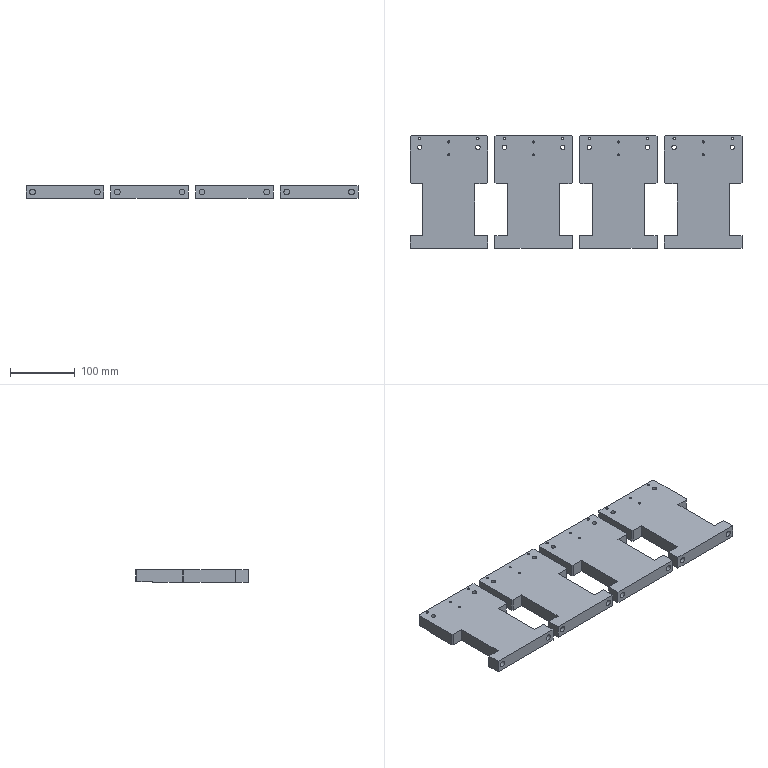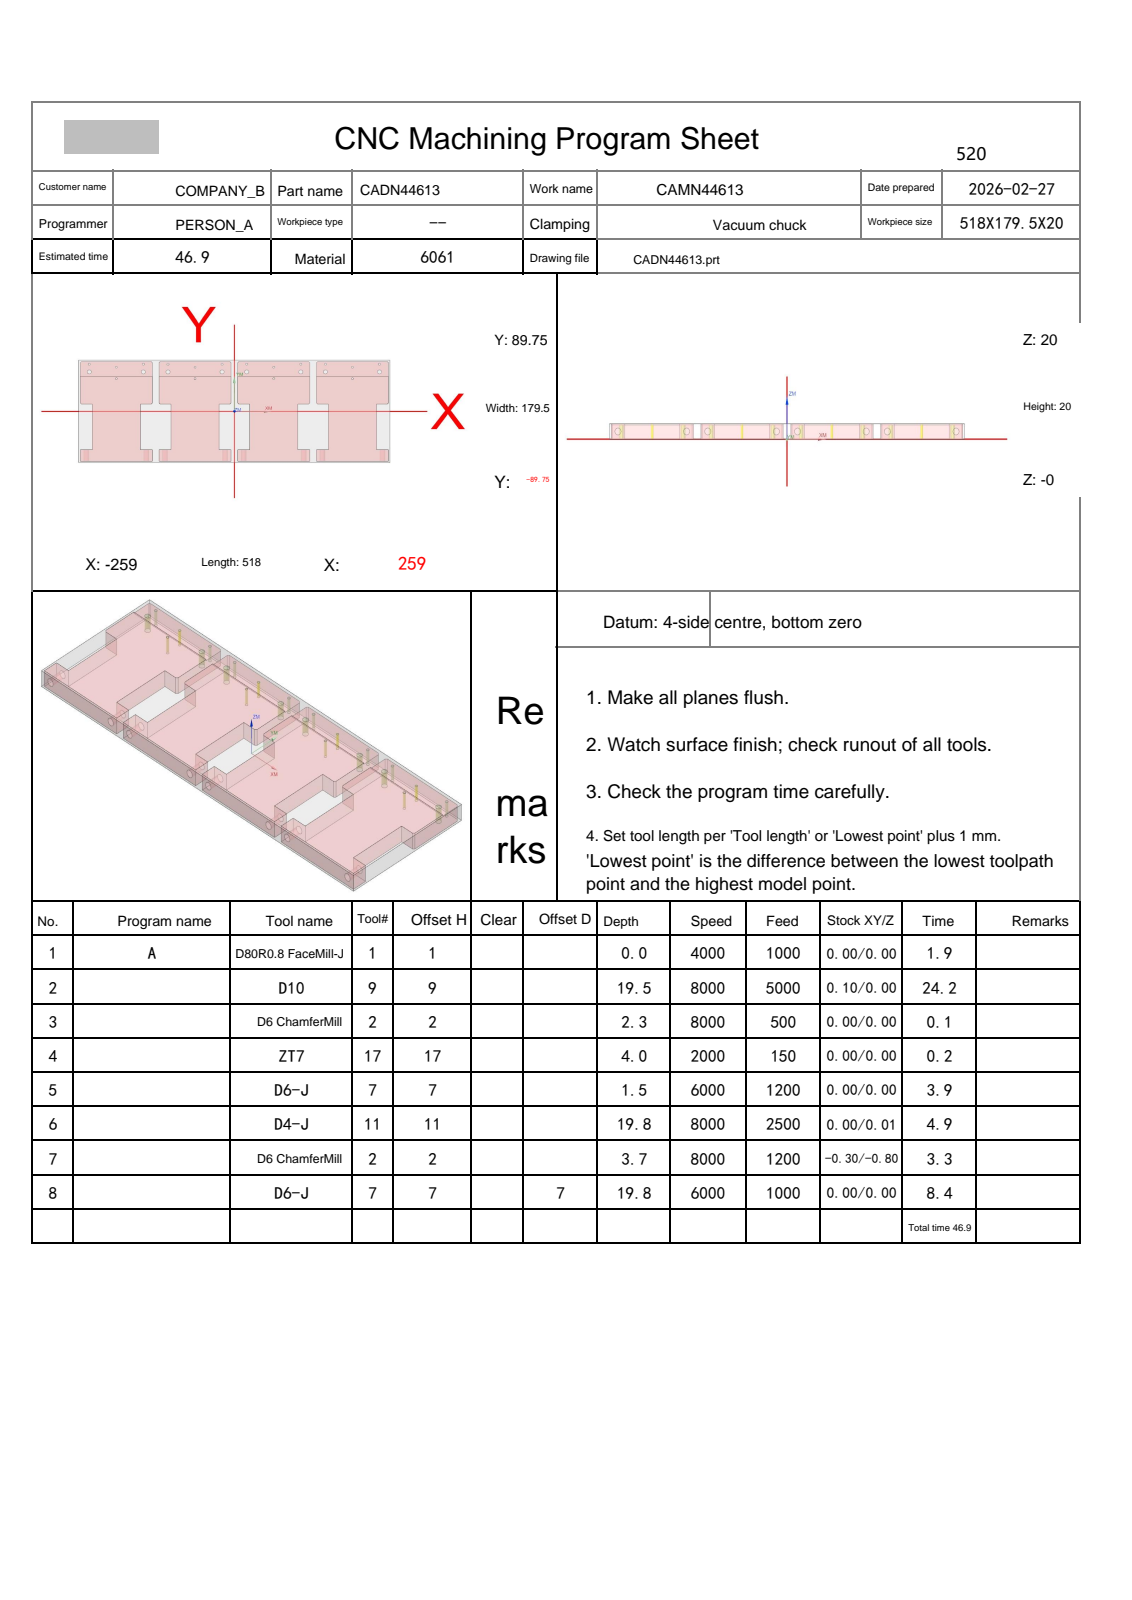NC program | NX | posted by the shop | part box 513 x 174.5 x 20 mm
Lines 4939 to 5164 of 36838:
N3 T02 M06
(D6 ChamferMill  D=6. R=0. H=02 ce=0.00 di=0.00)
G00 G90 G54 X-241.5 Y69.1 M03 S8000
G43 H02 Z50.
M08
G98 G81 X-241.5 Y69.1 Z17.7 R19.5 F500.
X-151.5
X-110.5
X-20.5
X20.5
X110.5
X151.5
X241.5
G80
G00 Z50.
G91 G28 Z0.0
M05
M09
G91 G28 Z0.0
M01
N4 T17 M06
(ZT7 D=7. DR_a=118 H=17)
G00 G90 G54 X-241.5 Y69.1 M03 S2000
G43 H17 Z50.
M08
G98 G83 X-241.5 Y69.1 Z16. R19.5 F150. Q2.
X-151.5
X-110.5
X-20.5
X20.5
X110.5
X151.5
X241.5
G80
G00 Z50.
G91 G28 Z0.0
M05
M09
G91 G28 Z0.0
M01
N5 T07 M06
(D6-J  D=6. R=0. H=07 ce=0.30 di=0.00)
G00 G90 G54 X196.5 Y93.25 M03 S6000
G43 H07 Z50.
M08
Z19.
G01 Z18.5 F1200.
Y87.85
X254.749
X257.1 Y85.499
Y64.4
X135.9
Y85.499
X138.251 Y87.85
X196.5
Y83.65
X252.9
Y68.6
X140.1
Y83.65
X196.5
Y79.45
X248.7
Y72.8
X144.3
Y79.45
X196.5
Y76.75
X246.
Y75.5
X147.
Y76.75
X196.5
X197.
Y80.35
Z19.
G00 Z50.
X65.5 Y93.25
Z19.
G01 Z18.5
Y87.85
X123.749
X126.1 Y85.499
Y64.4
X4.9
Y85.499
X7.251 Y87.85
X65.5
Y83.65
X121.9
Y68.6
X9.1
Y83.65
X65.5
Y79.45
X117.7
Y72.8
X13.3
Y79.45
X65.5
Y76.75
X115.
Y75.5
X16.
Y76.75
X65.5
X66.
Y80.35
Z19.
G00 Z50.
X-65.5 Y93.25
Z19.
G01 Z18.5
Y87.85
X-7.251
X-4.9 Y85.499
Y64.4
X-126.1
Y85.499
X-123.749 Y87.85
X-65.5
Y83.65
X-9.1
Y68.6
X-121.9
Y83.65
X-65.5
Y79.45
X-13.3
Y72.8
X-117.7
Y79.45
X-65.5
Y76.75
X-16.
Y75.5
X-115.
Y76.75
X-65.5
X-65.
Y80.35
Z19.
G00 Z50.
X-196.5 Y93.25
Z19.
G01 Z18.5
Y87.85
X-138.251
X-135.9 Y85.499
Y64.4
X-257.1
Y85.499
X-254.749 Y87.85
X-196.5
Y83.65
X-140.1
Y68.6
X-252.9
Y83.65
X-196.5
Y79.45
X-144.3
Y72.8
X-248.7
Y79.45
X-196.5
Y76.75
X-147.
Y75.5
X-246.
Y76.75
X-196.5
X-196.
Y80.35
Z19.
G00 Z50.
G00 G90 X132.8 Y65.2 M03 S6000
Z50.
Z19.005
G01 Z18.505 F1200.
G41 D07
Y65.1
G03 X133.8 Y64.1 I1. J0.0
G01 X259.2
G03 X260.2 Y65.1 I0.0 J1.
G01 G40 Y65.2
Z19.005
G00 Z50.
X1.8
Z19.005
G01 Z18.505
G41 D07
Y65.1
G03 X2.8 Y64.1 I1. J0.0
G01 X128.2
G03 X129.2 Y65.1 I0.0 J1.
G01 G40 Y65.2
Z19.005
G00 Z50.
X-129.2
Z19.005
G01 Z18.505
G41 D07
Y65.1
G03 X-128.2 Y64.1 I1. J0.0
G01 X-2.8
G03 X-1.8 Y65.1 I0.0 J1.
G01 G40 Y65.2
Z19.005
G00 Z50.
X-260.2
Z19.005
G01 Z18.505
G41 D07
Y65.1
G03 X-259.2 Y64.1 I1. J0.0
G01 X-133.8
G03 X-132.8 Y65.1 I0.0 J1.
G01 G40 Y65.2
Z19.005
G00 Z50.
G91 G28 Z0.0
M05
M09
G91 G28 Z0.0
M01